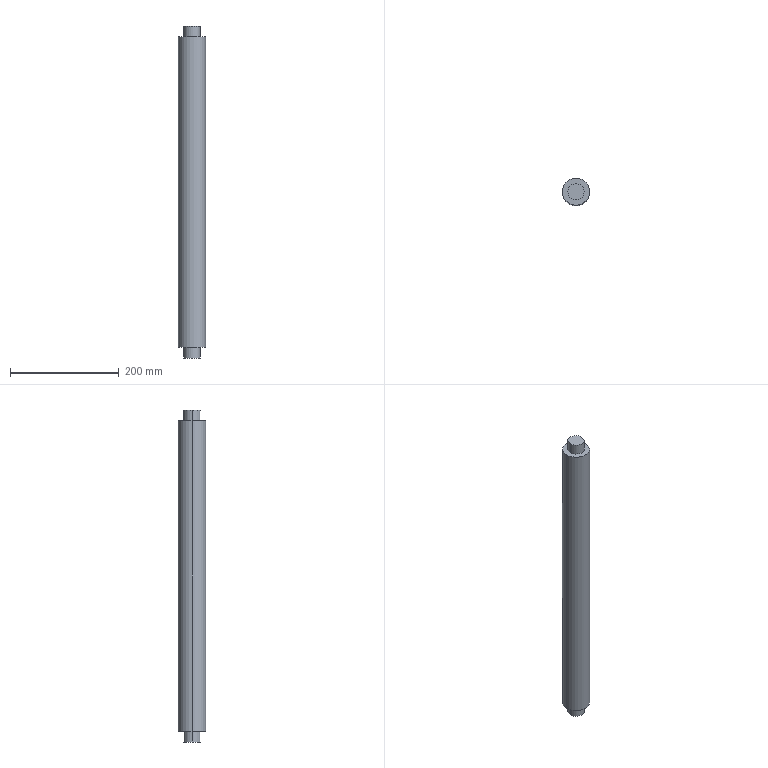Part | STEP file | 1 solid | 10 faces | box 50 x 50 x 610 mm | volume 1147467 mm3 | cylinder 6 | plane 4 | commonest cylinder face diameters 30 x4 50 x2
STEP:
#1=CARTESIAN_POINT('',(0.,0.,0.));
#2=DIRECTION('',(0.,0.,1.));
#3=DIRECTION('',(1.,0.,0.));
#4=AXIS2_PLACEMENT_3D('',#1,#2,#3);
#5=CARTESIAN_POINT('',(25.,0.,0.));
#6=VERTEX_POINT('',#5);
#7=CARTESIAN_POINT('',(-25.,0.,0.));
#8=VERTEX_POINT('',#7);
#9=CARTESIAN_POINT('',(0.,0.,0.));
#10=DIRECTION('',(0.,0.,1.));
#11=DIRECTION('',(1.,0.,0.));
#12=AXIS2_PLACEMENT_3D('',#9,#10,#11);
#13=CIRCLE('',#12,25.);
#14=CARTESIAN_POINT('',(0.,0.,0.));
#15=DIRECTION('',(0.,0.,1.));
#16=DIRECTION('',(1.,0.,0.));
#17=AXIS2_PLACEMENT_3D('',#14,#15,#16);
#18=CYLINDRICAL_SURFACE('',#17,25.);
#19=CARTESIAN_POINT('',(0.,0.));
#20=DIRECTION('',(1.,0.));
#21=VECTOR('',#20,1.);
#22=LINE('',#19,#21);
#23=(GEOMETRIC_REPRESENTATION_CONTEXT(2)PARAMETRIC_REPRESENTATION_CONTEXT()REPRESENTATION_CONTEXT('',''));
#24=DEFINITIONAL_REPRESENTATION('',(#22),#23);
#25=PCURVE('',#18,#24);
#26=CARTESIAN_POINT('',(0.,0.,0.));
#27=DIRECTION('',(0.,0.,1.));
#28=DIRECTION('',(1.,0.,0.));
#29=AXIS2_PLACEMENT_3D('',#26,#27,#28);
#30=PLANE('',#29);
#31=CARTESIAN_POINT('',(0.,0.));
#32=DIRECTION('',(1.,0.));
#33=AXIS2_PLACEMENT_2D('',#31,#32);
#34=CIRCLE('',#33,25.);
#35=(GEOMETRIC_REPRESENTATION_CONTEXT(2)PARAMETRIC_REPRESENTATION_CONTEXT()REPRESENTATION_CONTEXT('',''));
#36=DEFINITIONAL_REPRESENTATION('',(#34),#35);
#37=PCURVE('',#30,#36);
#38=SURFACE_CURVE('',#13,(#25,#37),.PCURVE_S1.);
#39=EDGE_CURVE('',#6,#8,#38,.T.);
#40=ORIENTED_EDGE('',*,*,#39,.T.);
#41=CARTESIAN_POINT('',(-25.,0.,570.));
#42=VERTEX_POINT('',#41);
#43=CARTESIAN_POINT('',(-25.,0.,0.));
#44=DIRECTION('',(0.,0.,1.));
#45=VECTOR('',#44,1.);
#46=LINE('',#43,#45);
#47=CARTESIAN_POINT('',(3.142,0.));
#48=DIRECTION('',(0.,1.));
#49=VECTOR('',#48,1.);
#50=LINE('',#47,#49);
#51=(GEOMETRIC_REPRESENTATION_CONTEXT(2)PARAMETRIC_REPRESENTATION_CONTEXT()REPRESENTATION_CONTEXT('',''));
#52=DEFINITIONAL_REPRESENTATION('',(#50),#51);
#53=PCURVE('',#18,#52);
#54=CARTESIAN_POINT('',(0.,0.,0.));
#55=DIRECTION('',(0.,0.,1.));
#56=DIRECTION('',(1.,0.,0.));
#57=AXIS2_PLACEMENT_3D('',#54,#55,#56);
#58=CYLINDRICAL_SURFACE('',#57,25.);
#59=CARTESIAN_POINT('',(3.142,0.));
#60=DIRECTION('',(0.,1.));
#61=VECTOR('',#60,1.);
#62=LINE('',#59,#61);
#63=(GEOMETRIC_REPRESENTATION_CONTEXT(2)PARAMETRIC_REPRESENTATION_CONTEXT()REPRESENTATION_CONTEXT('',''));
#64=DEFINITIONAL_REPRESENTATION('',(#62),#63);
#65=PCURVE('',#58,#64);
#66=SURFACE_CURVE('',#46,(#53,#65),.PCURVE_S1.);
#67=EDGE_CURVE('',#8,#42,#66,.T.);
#68=ORIENTED_EDGE('',*,*,#67,.T.);
#69=CARTESIAN_POINT('',(25.,0.,570.));
#70=VERTEX_POINT('',#69);
#71=CARTESIAN_POINT('',(0.,0.,570.));
#72=DIRECTION('',(0.,0.,-1.));
#73=DIRECTION('',(1.,0.,0.));
#74=AXIS2_PLACEMENT_3D('',#71,#72,#73);
#75=CIRCLE('',#74,25.);
#76=CARTESIAN_POINT('',(6.283,570.));
#77=DIRECTION('',(-1.,0.));
#78=VECTOR('',#77,1.);
#79=LINE('',#76,#78);
#80=(GEOMETRIC_REPRESENTATION_CONTEXT(2)PARAMETRIC_REPRESENTATION_CONTEXT()REPRESENTATION_CONTEXT('',''));
#81=DEFINITIONAL_REPRESENTATION('',(#79),#80);
#82=PCURVE('',#18,#81);
#83=CARTESIAN_POINT('',(0.,0.,570.));
#84=DIRECTION('',(0.,0.,1.));
#85=DIRECTION('',(1.,0.,0.));
#86=AXIS2_PLACEMENT_3D('',#83,#84,#85);
#87=PLANE('',#86);
#88=CARTESIAN_POINT('',(25.,0.));
#89=CARTESIAN_POINT('',(25.,-43.301));
#90=CARTESIAN_POINT('',(-12.5,-21.651));
#91=CARTESIAN_POINT('',(-50.,0.));
#92=CARTESIAN_POINT('',(-12.5,21.651));
#93=CARTESIAN_POINT('',(25.,43.301));
#94=CARTESIAN_POINT('',(25.,0.));
#95=(BOUNDED_CURVE()B_SPLINE_CURVE(2,(#88,#89,#90,#91,#92,#93,#94),.UNSPECIFIED.,.T.,.F.)B_SPLINE_CURVE_WITH_KNOTS((1,2,2,2,2,1),(-2.094,0.,2.094,4.189,6.283,8.378),.UNSPECIFIED.)CURVE()GEOMETRIC_REPRESENTATION_ITEM()RATIONAL_B_SPLINE_CURVE((1.,0.5,1.,0.5,1.,0.5,1.))REPRESENTATION_ITEM(''));
#96=(GEOMETRIC_REPRESENTATION_CONTEXT(2)PARAMETRIC_REPRESENTATION_CONTEXT()REPRESENTATION_CONTEXT('',''));
#97=DEFINITIONAL_REPRESENTATION('',(#95),#96);
#98=PCURVE('',#87,#97);
#99=SURFACE_CURVE('',#75,(#82,#98),.PCURVE_S1.);
#100=EDGE_CURVE('',#42,#70,#99,.T.);
#101=ORIENTED_EDGE('',*,*,#100,.T.);
#102=CARTESIAN_POINT('',(25.,0.,0.));
#103=DIRECTION('',(0.,0.,1.));
#104=VECTOR('',#103,1.);
#105=LINE('',#102,#104);
#106=CARTESIAN_POINT('',(0.,0.));
#107=DIRECTION('',(0.,1.));
#108=VECTOR('',#107,1.);
#109=LINE('',#106,#108);
#110=(GEOMETRIC_REPRESENTATION_CONTEXT(2)PARAMETRIC_REPRESENTATION_CONTEXT()REPRESENTATION_CONTEXT('',''));
#111=DEFINITIONAL_REPRESENTATION('',(#109),#110);
#112=PCURVE('',#18,#111);
#113=CARTESIAN_POINT('',(6.283,0.));
#114=DIRECTION('',(0.,1.));
#115=VECTOR('',#114,1.);
#116=LINE('',#113,#115);
#117=(GEOMETRIC_REPRESENTATION_CONTEXT(2)PARAMETRIC_REPRESENTATION_CONTEXT()REPRESENTATION_CONTEXT('',''));
#118=DEFINITIONAL_REPRESENTATION('',(#116),#117);
#119=PCURVE('',#58,#118);
#120=SURFACE_CURVE('',#105,(#112,#119),.PCURVE_S1.);
#121=EDGE_CURVE('',#6,#70,#120,.T.);
#122=ORIENTED_EDGE('',*,*,#121,.F.);
#123=EDGE_LOOP('',(#40,#68,#101,#122));
#124=FACE_BOUND('',#123,.T.);
#125=ADVANCED_FACE('',(#124),#18,.T.);
#126=CARTESIAN_POINT('',(-15.,0.,0.));
#127=VERTEX_POINT('',#126);
#128=CARTESIAN_POINT('',(15.,0.,0.));
#129=VERTEX_POINT('',#128);
#130=CARTESIAN_POINT('',(0.,0.,0.));
#131=DIRECTION('',(0.,0.,-1.));
#132=DIRECTION('',(-1.,0.,0.));
#133=AXIS2_PLACEMENT_3D('',#130,#131,#132);
#134=CIRCLE('',#133,15.);
#135=CARTESIAN_POINT('',(0.,0.,0.));
#136=DIRECTION('',(0.,0.,-1.));
#137=DIRECTION('',(-1.,0.,0.));
#138=AXIS2_PLACEMENT_3D('',#135,#136,#137);
#139=CYLINDRICAL_SURFACE('',#138,15.);
#140=CARTESIAN_POINT('',(0.,0.));
#141=DIRECTION('',(1.,0.));
#142=VECTOR('',#141,1.);
#143=LINE('',#140,#142);
#144=(GEOMETRIC_REPRESENTATION_CONTEXT(2)PARAMETRIC_REPRESENTATION_CONTEXT()REPRESENTATION_CONTEXT('',''));
#145=DEFINITIONAL_REPRESENTATION('',(#143),#144);
#146=PCURVE('',#139,#145);
#147=CARTESIAN_POINT('',(-15.,0.));
#148=CARTESIAN_POINT('',(-15.,25.981));
#149=CARTESIAN_POINT('',(7.5,12.99));
#150=CARTESIAN_POINT('',(30.,0.));
#151=CARTESIAN_POINT('',(7.5,-12.99));
#152=CARTESIAN_POINT('',(-15.,-25.981));
#153=CARTESIAN_POINT('',(-15.,0.));
#154=(BOUNDED_CURVE()B_SPLINE_CURVE(2,(#147,#148,#149,#150,#151,#152,#153),.UNSPECIFIED.,.T.,.F.)B_SPLINE_CURVE_WITH_KNOTS((1,2,2,2,2,1),(-2.094,0.,2.094,4.189,6.283,8.378),.UNSPECIFIED.)CURVE()GEOMETRIC_REPRESENTATION_ITEM()RATIONAL_B_SPLINE_CURVE((1.,0.5,1.,0.5,1.,0.5,1.))REPRESENTATION_ITEM(''));
#155=(GEOMETRIC_REPRESENTATION_CONTEXT(2)PARAMETRIC_REPRESENTATION_CONTEXT()REPRESENTATION_CONTEXT('',''));
#156=DEFINITIONAL_REPRESENTATION('',(#154),#155);
#157=PCURVE('',#30,#156);
#158=SURFACE_CURVE('',#134,(#146,#157),.PCURVE_S1.);
#159=EDGE_CURVE('',#127,#129,#158,.T.);
#160=ORIENTED_EDGE('',*,*,#159,.T.);
#161=CARTESIAN_POINT('',(15.,0.,-20.));
#162=VERTEX_POINT('',#161);
#163=CARTESIAN_POINT('',(15.,0.,0.));
#164=DIRECTION('',(0.,0.,-1.));
#165=VECTOR('',#164,1.);
#166=LINE('',#163,#165);
#167=CARTESIAN_POINT('',(3.142,0.));
#168=DIRECTION('',(0.,1.));
#169=VECTOR('',#168,1.);
#170=LINE('',#167,#169);
#171=(GEOMETRIC_REPRESENTATION_CONTEXT(2)PARAMETRIC_REPRESENTATION_CONTEXT()REPRESENTATION_CONTEXT('',''));
#172=DEFINITIONAL_REPRESENTATION('',(#170),#171);
#173=PCURVE('',#139,#172);
#174=CARTESIAN_POINT('',(0.,0.,0.));
#175=DIRECTION('',(0.,0.,-1.));
#176=DIRECTION('',(-1.,0.,0.));
#177=AXIS2_PLACEMENT_3D('',#174,#175,#176);
#178=CYLINDRICAL_SURFACE('',#177,15.);
#179=CARTESIAN_POINT('',(3.142,0.));
#180=DIRECTION('',(0.,1.));
#181=VECTOR('',#180,1.);
#182=LINE('',#179,#181);
#183=(GEOMETRIC_REPRESENTATION_CONTEXT(2)PARAMETRIC_REPRESENTATION_CONTEXT()REPRESENTATION_CONTEXT('',''));
#184=DEFINITIONAL_REPRESENTATION('',(#182),#183);
#185=PCURVE('',#178,#184);
#186=SURFACE_CURVE('',#166,(#173,#185),.PCURVE_S1.);
#187=EDGE_CURVE('',#129,#162,#186,.T.);
#188=ORIENTED_EDGE('',*,*,#187,.T.);
#189=CARTESIAN_POINT('',(-15.,0.,-20.));
#190=VERTEX_POINT('',#189);
#191=CARTESIAN_POINT('',(0.,0.,-20.));
#192=DIRECTION('',(0.,0.,1.));
#193=DIRECTION('',(-1.,0.,0.));
#194=AXIS2_PLACEMENT_3D('',#191,#192,#193);
#195=CIRCLE('',#194,15.);
#196=CARTESIAN_POINT('',(6.283,20.));
#197=DIRECTION('',(-1.,0.));
#198=VECTOR('',#197,1.);
#199=LINE('',#196,#198);
#200=(GEOMETRIC_REPRESENTATION_CONTEXT(2)PARAMETRIC_REPRESENTATION_CONTEXT()REPRESENTATION_CONTEXT('',''));
#201=DEFINITIONAL_REPRESENTATION('',(#199),#200);
#202=PCURVE('',#139,#201);
#203=CARTESIAN_POINT('',(0.,0.,-20.));
#204=DIRECTION('',(0.,0.,1.));
#205=DIRECTION('',(1.,0.,0.));
#206=AXIS2_PLACEMENT_3D('',#203,#204,#205);
#207=PLANE('',#206);
#208=CARTESIAN_POINT('',(0.,0.));
#209=DIRECTION('',(-1.,0.));
#210=AXIS2_PLACEMENT_2D('',#208,#209);
#211=CIRCLE('',#210,15.);
#212=(GEOMETRIC_REPRESENTATION_CONTEXT(2)PARAMETRIC_REPRESENTATION_CONTEXT()REPRESENTATION_CONTEXT('',''));
#213=DEFINITIONAL_REPRESENTATION('',(#211),#212);
#214=PCURVE('',#207,#213);
#215=SURFACE_CURVE('',#195,(#202,#214),.PCURVE_S1.);
#216=EDGE_CURVE('',#162,#190,#215,.T.);
#217=ORIENTED_EDGE('',*,*,#216,.T.);
#218=CARTESIAN_POINT('',(-15.,0.,0.));
#219=DIRECTION('',(0.,0.,-1.));
#220=VECTOR('',#219,1.);
#221=LINE('',#218,#220);
#222=CARTESIAN_POINT('',(0.,0.));
#223=DIRECTION('',(0.,1.));
#224=VECTOR('',#223,1.);
#225=LINE('',#222,#224);
#226=(GEOMETRIC_REPRESENTATION_CONTEXT(2)PARAMETRIC_REPRESENTATION_CONTEXT()REPRESENTATION_CONTEXT('',''));
#227=DEFINITIONAL_REPRESENTATION('',(#225),#226);
#228=PCURVE('',#139,#227);
#229=CARTESIAN_POINT('',(6.283,0.));
#230=DIRECTION('',(0.,1.));
#231=VECTOR('',#230,1.);
#232=LINE('',#229,#231);
#233=(GEOMETRIC_REPRESENTATION_CONTEXT(2)PARAMETRIC_REPRESENTATION_CONTEXT()REPRESENTATION_CONTEXT('',''));
#234=DEFINITIONAL_REPRESENTATION('',(#232),#233);
#235=PCURVE('',#178,#234);
#236=SURFACE_CURVE('',#221,(#228,#235),.PCURVE_S1.);
#237=EDGE_CURVE('',#127,#190,#236,.T.);
#238=ORIENTED_EDGE('',*,*,#237,.F.);
#239=EDGE_LOOP('',(#160,#188,#217,#238));
#240=FACE_BOUND('',#239,.T.);
#241=ADVANCED_FACE('',(#240),#139,.T.);
#242=CARTESIAN_POINT('',(-15.,0.,570.));
#243=VERTEX_POINT('',#242);
#244=CARTESIAN_POINT('',(15.,0.,570.));
#245=VERTEX_POINT('',#244);
#246=CARTESIAN_POINT('',(0.,0.,570.));
#247=DIRECTION('',(0.,0.,-1.));
#248=DIRECTION('',(1.,0.,0.));
#249=AXIS2_PLACEMENT_3D('',#246,#247,#248);
#250=CIRCLE('',#249,15.);
#251=CARTESIAN_POINT('',(0.,0.,570.));
#252=DIRECTION('',(0.,0.,1.));
#253=DIRECTION('',(1.,0.,0.));
#254=AXIS2_PLACEMENT_3D('',#251,#252,#253);
#255=CYLINDRICAL_SURFACE('',#254,15.);
#256=CARTESIAN_POINT('',(6.283,0.));
#257=DIRECTION('',(-1.,0.));
#258=VECTOR('',#257,1.);
#259=LINE('',#256,#258);
#260=(GEOMETRIC_REPRESENTATION_CONTEXT(2)PARAMETRIC_REPRESENTATION_CONTEXT()REPRESENTATION_CONTEXT('',''));
#261=DEFINITIONAL_REPRESENTATION('',(#259),#260);
#262=PCURVE('',#255,#261);
#263=CARTESIAN_POINT('',(15.,0.));
#264=CARTESIAN_POINT('',(15.,-25.981));
#265=CARTESIAN_POINT('',(-7.5,-12.99));
#266=CARTESIAN_POINT('',(-30.,0.));
#267=CARTESIAN_POINT('',(-7.5,12.99));
#268=CARTESIAN_POINT('',(15.,25.981));
#269=CARTESIAN_POINT('',(15.,0.));
#270=(BOUNDED_CURVE()B_SPLINE_CURVE(2,(#263,#264,#265,#266,#267,#268,#269),.UNSPECIFIED.,.T.,.F.)B_SPLINE_CURVE_WITH_KNOTS((1,2,2,2,2,1),(-2.094,0.,2.094,4.189,6.283,8.378),.UNSPECIFIED.)CURVE()GEOMETRIC_REPRESENTATION_ITEM()RATIONAL_B_SPLINE_CURVE((1.,0.5,1.,0.5,1.,0.5,1.))REPRESENTATION_ITEM(''));
#271=(GEOMETRIC_REPRESENTATION_CONTEXT(2)PARAMETRIC_REPRESENTATION_CONTEXT()REPRESENTATION_CONTEXT('',''));
#272=DEFINITIONAL_REPRESENTATION('',(#270),#271);
#273=PCURVE('',#87,#272);
#274=SURFACE_CURVE('',#250,(#262,#273),.PCURVE_S1.);
#275=EDGE_CURVE('',#243,#245,#274,.T.);
#276=ORIENTED_EDGE('',*,*,#275,.F.);
#277=CARTESIAN_POINT('',(-15.,0.,590.));
#278=VERTEX_POINT('',#277);
#279=CARTESIAN_POINT('',(-15.,0.,570.));
#280=DIRECTION('',(0.,0.,1.));
#281=VECTOR('',#280,1.);
#282=LINE('',#279,#281);
#283=CARTESIAN_POINT('',(3.142,0.));
#284=DIRECTION('',(0.,1.));
#285=VECTOR('',#284,1.);
#286=LINE('',#283,#285);
#287=(GEOMETRIC_REPRESENTATION_CONTEXT(2)PARAMETRIC_REPRESENTATION_CONTEXT()REPRESENTATION_CONTEXT('',''));
#288=DEFINITIONAL_REPRESENTATION('',(#286),#287);
#289=PCURVE('',#255,#288);
#290=CARTESIAN_POINT('',(0.,0.,570.));
#291=DIRECTION('',(0.,0.,1.));
#292=DIRECTION('',(1.,0.,0.));
#293=AXIS2_PLACEMENT_3D('',#290,#291,#292);
#294=CYLINDRICAL_SURFACE('',#293,15.);
#295=CARTESIAN_POINT('',(3.142,0.));
#296=DIRECTION('',(0.,1.));
#297=VECTOR('',#296,1.);
#298=LINE('',#295,#297);
#299=(GEOMETRIC_REPRESENTATION_CONTEXT(2)PARAMETRIC_REPRESENTATION_CONTEXT()REPRESENTATION_CONTEXT('',''));
#300=DEFINITIONAL_REPRESENTATION('',(#298),#299);
#301=PCURVE('',#294,#300);
#302=SURFACE_CURVE('',#282,(#289,#301),.PCURVE_S1.);
#303=EDGE_CURVE('',#243,#278,#302,.T.);
#304=ORIENTED_EDGE('',*,*,#303,.T.);
#305=CARTESIAN_POINT('',(15.,0.,590.));
#306=VERTEX_POINT('',#305);
#307=CARTESIAN_POINT('',(0.,0.,590.));
#308=DIRECTION('',(0.,0.,-1.));
#309=DIRECTION('',(1.,0.,0.));
#310=AXIS2_PLACEMENT_3D('',#307,#308,#309);
#311=CIRCLE('',#310,15.);
#312=CARTESIAN_POINT('',(6.283,20.));
#313=DIRECTION('',(-1.,0.));
#314=VECTOR('',#313,1.);
#315=LINE('',#312,#314);
#316=(GEOMETRIC_REPRESENTATION_CONTEXT(2)PARAMETRIC_REPRESENTATION_CONTEXT()REPRESENTATION_CONTEXT('',''));
#317=DEFINITIONAL_REPRESENTATION('',(#315),#316);
#318=PCURVE('',#255,#317);
#319=CARTESIAN_POINT('',(0.,0.,590.));
#320=DIRECTION('',(0.,0.,1.));
#321=DIRECTION('',(1.,0.,0.));
#322=AXIS2_PLACEMENT_3D('',#319,#320,#321);
#323=PLANE('',#322);
#324=CARTESIAN_POINT('',(15.,0.));
#325=CARTESIAN_POINT('',(15.,-25.981));
#326=CARTESIAN_POINT('',(-7.5,-12.99));
#327=CARTESIAN_POINT('',(-30.,0.));
#328=CARTESIAN_POINT('',(-7.5,12.99));
#329=CARTESIAN_POINT('',(15.,25.981));
#330=CARTESIAN_POINT('',(15.,0.));
#331=(BOUNDED_CURVE()B_SPLINE_CURVE(2,(#324,#325,#326,#327,#328,#329,#330),.UNSPECIFIED.,.T.,.F.)B_SPLINE_CURVE_WITH_KNOTS((1,2,2,2,2,1),(-2.094,0.,2.094,4.189,6.283,8.378),.UNSPECIFIED.)CURVE()GEOMETRIC_REPRESENTATION_ITEM()RATIONAL_B_SPLINE_CURVE((1.,0.5,1.,0.5,1.,0.5,1.))REPRESENTATION_ITEM(''));
#332=(GEOMETRIC_REPRESENTATION_CONTEXT(2)PARAMETRIC_REPRESENTATION_CONTEXT()REPRESENTATION_CONTEXT('',''));
#333=DEFINITIONAL_REPRESENTATION('',(#331),#332);
#334=PCURVE('',#323,#333);
#335=SURFACE_CURVE('',#311,(#318,#334),.PCURVE_S1.);
#336=EDGE_CURVE('',#278,#306,#335,.T.);
#337=ORIENTED_EDGE('',*,*,#336,.T.);
#338=CARTESIAN_POINT('',(15.,0.,570.));
#339=DIRECTION('',(0.,0.,1.));
#340=VECTOR('',#339,1.);
#341=LINE('',#338,#340);
#342=CARTESIAN_POINT('',(0.,0.));
#343=DIRECTION('',(0.,1.));
#344=VECTOR('',#343,1.);
#345=LINE('',#342,#344);
#346=(GEOMETRIC_REPRESENTATION_CONTEXT(2)PARAMETRIC_REPRESENTATION_CONTEXT()REPRESENTATION_CONTEXT('',''));
#347=DEFINITIONAL_REPRESENTATION('',(#345),#346);
#348=PCURVE('',#255,#347);
#349=CARTESIAN_POINT('',(6.283,0.));
#350=DIRECTION('',(0.,1.));
#351=VECTOR('',#350,1.);
#352=LINE('',#349,#351);
#353=(GEOMETRIC_REPRESENTATION_CONTEXT(2)PARAMETRIC_REPRESENTATION_CONTEXT()REPRESENTATION_CONTEXT('',''));
#354=DEFINITIONAL_REPRESENTATION('',(#352),#353);
#355=PCURVE('',#294,#354);
#356=SURFACE_CURVE('',#341,(#348,#355),.PCURVE_S1.);
#357=EDGE_CURVE('',#245,#306,#356,.T.);
#358=ORIENTED_EDGE('',*,*,#357,.F.);
#359=EDGE_LOOP('',(#276,#304,#337,#358));
#360=FACE_BOUND('',#359,.T.);
#361=ADVANCED_FACE('',(#360),#255,.T.);
#362=ORIENTED_EDGE('',*,*,#67,.F.);
#363=CARTESIAN_POINT('',(0.,0.,0.));
#364=DIRECTION('',(0.,0.,1.));
#365=DIRECTION('',(1.,0.,0.));
#366=AXIS2_PLACEMENT_3D('',#363,#364,#365);
#367=CIRCLE('',#366,25.);
#368=CARTESIAN_POINT('',(0.,0.));
#369=DIRECTION('',(1.,0.));
#370=VECTOR('',#369,1.);
#371=LINE('',#368,#370);
#372=(GEOMETRIC_REPRESENTATION_CONTEXT(2)PARAMETRIC_REPRESENTATION_CONTEXT()REPRESENTATION_CONTEXT('',''));
#373=DEFINITIONAL_REPRESENTATION('',(#371),#372);
#374=PCURVE('',#58,#373);
#375=CARTESIAN_POINT('',(0.,0.));
#376=DIRECTION('',(1.,0.));
#377=AXIS2_PLACEMENT_2D('',#375,#376);
#378=CIRCLE('',#377,25.);
#379=(GEOMETRIC_REPRESENTATION_CONTEXT(2)PARAMETRIC_REPRESENTATION_CONTEXT()REPRESENTATION_CONTEXT('',''));
#380=DEFINITIONAL_REPRESENTATION('',(#378),#379);
#381=PCURVE('',#30,#380);
#382=SURFACE_CURVE('',#367,(#374,#381),.PCURVE_S1.);
#383=EDGE_CURVE('',#8,#6,#382,.T.);
#384=ORIENTED_EDGE('',*,*,#383,.T.);
#385=ORIENTED_EDGE('',*,*,#121,.T.);
#386=CARTESIAN_POINT('',(0.,0.,570.));
#387=DIRECTION('',(0.,0.,-1.));
#388=DIRECTION('',(1.,0.,0.));
#389=AXIS2_PLACEMENT_3D('',#386,#387,#388);
#390=CIRCLE('',#389,25.);
#391=CARTESIAN_POINT('',(6.283,570.));
#392=DIRECTION('',(-1.,0.));
#393=VECTOR('',#392,1.);
#394=LINE('',#391,#393);
#395=(GEOMETRIC_REPRESENTATION_CONTEXT(2)PARAMETRIC_REPRESENTATION_CONTEXT()REPRESENTATION_CONTEXT('',''));
#396=DEFINITIONAL_REPRESENTATION('',(#394),#395);
#397=PCURVE('',#58,#396);
#398=CARTESIAN_POINT('',(25.,0.));
#399=CARTESIAN_POINT('',(25.,-43.301));
#400=CARTESIAN_POINT('',(-12.5,-21.651));
#401=CARTESIAN_POINT('',(-50.,0.));
#402=CARTESIAN_POINT('',(-12.5,21.651));
#403=CARTESIAN_POINT('',(25.,43.301));
#404=CARTESIAN_POINT('',(25.,0.));
#405=(BOUNDED_CURVE()B_SPLINE_CURVE(2,(#398,#399,#400,#401,#402,#403,#404),.UNSPECIFIED.,.T.,.F.)B_SPLINE_CURVE_WITH_KNOTS((1,2,2,2,2,1),(-2.094,0.,2.094,4.189,6.283,8.378),.UNSPECIFIED.)CURVE()GEOMETRIC_REPRESENTATION_ITEM()RATIONAL_B_SPLINE_CURVE((1.,0.5,1.,0.5,1.,0.5,1.))REPRESENTATION_ITEM(''));
#406=(GEOMETRIC_REPRESENTATION_CONTEXT(2)PARAMETRIC_REPRESENTATION_CONTEXT()REPRESENTATION_CONTEXT('',''));
#407=DEFINITIONAL_REPRESENTATION('',(#405),#406);
#408=PCURVE('',#87,#407);
#409=SURFACE_CURVE('',#390,(#397,#408),.PCURVE_S1.);
#410=EDGE_CURVE('',#70,#42,#409,.T.);
#411=ORIENTED_EDGE('',*,*,#410,.T.);
#412=EDGE_LOOP('',(#362,#384,#385,#411));
#413=FACE_BOUND('',#412,.T.);
#414=ADVANCED_FACE('',(#413),#58,.T.);
#415=ORIENTED_EDGE('',*,*,#39,.F.);
#416=ORIENTED_EDGE('',*,*,#383,.F.);
#417=EDGE_LOOP('',(#415,#416));
#418=FACE_BOUND('',#417,.T.);
#419=ORIENTED_EDGE('',*,*,#159,.F.);
#420=CARTESIAN_POINT('',(0.,0.,0.));
#421=DIRECTION('',(0.,0.,-1.));
#422=DIRECTION('',(-1.,0.,0.));
#423=AXIS2_PLACEMENT_3D('',#420,#421,#422);
#424=CIRCLE('',#423,15.);
#425=CARTESIAN_POINT('',(-15.,0.));
#426=CARTESIAN_POINT('',(-15.,25.981));
#427=CARTESIAN_POINT('',(7.5,12.99));
#428=CARTESIAN_POINT('',(30.,0.));
#429=CARTESIAN_POINT('',(7.5,-12.99));
#430=CARTESIAN_POINT('',(-15.,-25.981));
#431=CARTESIAN_POINT('',(-15.,0.));
#432=(BOUNDED_CURVE()B_SPLINE_CURVE(2,(#425,#426,#427,#428,#429,#430,#431),.UNSPECIFIED.,.T.,.F.)B_SPLINE_CURVE_WITH_KNOTS((1,2,2,2,2,1),(-2.094,0.,2.094,4.189,6.283,8.378),.UNSPECIFIED.)CURVE()GEOMETRIC_REPRESENTATION_ITEM()RATIONAL_B_SPLINE_CURVE((1.,0.5,1.,0.5,1.,0.5,1.))REPRESENTATION_ITEM(''));
#433=(GEOMETRIC_REPRESENTATION_CONTEXT(2)PARAMETRIC_REPRESENTATION_CONTEXT()REPRESENTATION_CONTEXT('',''));
#434=DEFINITIONAL_REPRESENTATION('',(#432),#433);
#435=PCURVE('',#30,#434);
#436=CARTESIAN_POINT('',(0.,0.));
#437=DIRECTION('',(1.,0.));
#438=VECTOR('',#437,1.);
#439=LINE('',#436,#438);
#440=(GEOMETRIC_REPRESENTATION_CONTEXT(2)PARAMETRIC_REPRESENTATION_CONTEXT()REPRESENTATION_CONTEXT('',''));
#441=DEFINITIONAL_REPRESENTATION('',(#439),#440);
#442=PCURVE('',#178,#441);
#443=SURFACE_CURVE('',#424,(#435,#442),.PCURVE_S1.);
#444=EDGE_CURVE('',#129,#127,#443,.T.);
#445=ORIENTED_EDGE('',*,*,#444,.F.);
#446=EDGE_LOOP('',(#419,#445));
#447=FACE_BOUND('',#446,.T.);
#448=ADVANCED_FACE('',(#418,#447),#30,.F.);
#449=ORIENTED_EDGE('',*,*,#410,.F.);
#450=ORIENTED_EDGE('',*,*,#100,.F.);
#451=EDGE_LOOP('',(#449,#450));
#452=FACE_BOUND('',#451,.T.);
#453=CARTESIAN_POINT('',(0.,0.,570.));
#454=DIRECTION('',(0.,0.,-1.));
#455=DIRECTION('',(1.,0.,0.));
#456=AXIS2_PLACEMENT_3D('',#453,#454,#455);
#457=CIRCLE('',#456,15.);
#458=CARTESIAN_POINT('',(15.,0.));
#459=CARTESIAN_POINT('',(15.,-25.981));
#460=CARTESIAN_POINT('',(-7.5,-12.99));
#461=CARTESIAN_POINT('',(-30.,0.));
#462=CARTESIAN_POINT('',(-7.5,12.99));
#463=CARTESIAN_POINT('',(15.,25.981));
#464=CARTESIAN_POINT('',(15.,0.));
#465=(BOUNDED_CURVE()B_SPLINE_CURVE(2,(#458,#459,#460,#461,#462,#463,#464),.UNSPECIFIED.,.T.,.F.)B_SPLINE_CURVE_WITH_KNOTS((1,2,2,2,2,1),(-2.094,0.,2.094,4.189,6.283,8.378),.UNSPECIFIED.)CURVE()GEOMETRIC_REPRESENTATION_ITEM()RATIONAL_B_SPLINE_CURVE((1.,0.5,1.,0.5,1.,0.5,1.))REPRESENTATION_ITEM(''));
#466=(GEOMETRIC_REPRESENTATION_CONTEXT(2)PARAMETRIC_REPRESENTATION_CONTEXT()REPRESENTATION_CONTEXT('',''));
#467=DEFINITIONAL_REPRESENTATION('',(#465),#466);
#468=PCURVE('',#87,#467);
#469=CARTESIAN_POINT('',(6.283,0.));
#470=DIRECTION('',(-1.,0.));
#471=VECTOR('',#470,1.);
#472=LINE('',#469,#471);
#473=(GEOMETRIC_REPRESENTATION_CONTEXT(2)PARAMETRIC_REPRESENTATION_CONTEXT()REPRESENTATION_CONTEXT('',''));
#474=DEFINITIONAL_REPRESENTATION('',(#472),#473);
#475=PCURVE('',#294,#474);
#476=SURFACE_CURVE('',#457,(#468,#475),.PCURVE_S1.);
#477=EDGE_CURVE('',#245,#243,#476,.T.);
#478=ORIENTED_EDGE('',*,*,#477,.T.);
#479=ORIENTED_EDGE('',*,*,#275,.T.);
#480=EDGE_LOOP('',(#478,#479));
#481=FACE_BOUND('',#480,.T.);
#482=ADVANCED_FACE('',(#452,#481),#87,.T.);
#483=ORIENTED_EDGE('',*,*,#187,.F.);
#484=ORIENTED_EDGE('',*,*,#444,.T.);
#485=ORIENTED_EDGE('',*,*,#237,.T.);
#486=CARTESIAN_POINT('',(0.,0.,-20.));
#487=DIRECTION('',(0.,0.,1.));
#488=DIRECTION('',(-1.,0.,0.));
#489=AXIS2_PLACEMENT_3D('',#486,#487,#488);
#490=CIRCLE('',#489,15.);
#491=CARTESIAN_POINT('',(6.283,20.));
#492=DIRECTION('',(-1.,0.));
#493=VECTOR('',#492,1.);
#494=LINE('',#491,#493);
#495=(GEOMETRIC_REPRESENTATION_CONTEXT(2)PARAMETRIC_REPRESENTATION_CONTEXT()REPRESENTATION_CONTEXT('',''));
#496=DEFINITIONAL_REPRESENTATION('',(#494),#495);
#497=PCURVE('',#178,#496);
#498=CARTESIAN_POINT('',(0.,0.));
#499=DIRECTION('',(-1.,0.));
#500=AXIS2_PLACEMENT_2D('',#498,#499);
#501=CIRCLE('',#500,15.);
#502=(GEOMETRIC_REPRESENTATION_CONTEXT(2)PARAMETRIC_REPRESENTATION_CONTEXT()REPRESENTATION_CONTEXT('',''));
#503=DEFINITIONAL_REPRESENTATION('',(#501),#502);
#504=PCURVE('',#207,#503);
#505=SURFACE_CURVE('',#490,(#497,#504),.PCURVE_S1.);
#506=EDGE_CURVE('',#190,#162,#505,.T.);
#507=ORIENTED_EDGE('',*,*,#506,.T.);
#508=EDGE_LOOP('',(#483,#484,#485,#507));
#509=FACE_BOUND('',#508,.T.);
#510=ADVANCED_FACE('',(#509),#178,.T.);
#511=ORIENTED_EDGE('',*,*,#303,.F.);
#512=ORIENTED_EDGE('',*,*,#477,.F.);
#513=ORIENTED_EDGE('',*,*,#357,.T.);
#514=CARTESIAN_POINT('',(0.,0.,590.));
#515=DIRECTION('',(0.,0.,-1.));
#516=DIRECTION('',(1.,0.,0.));
#517=AXIS2_PLACEMENT_3D('',#514,#515,#516);
#518=CIRCLE('',#517,15.);
#519=CARTESIAN_POINT('',(6.283,20.));
#520=DIRECTION('',(-1.,0.));
#521=VECTOR('',#520,1.);
#522=LINE('',#519,#521);
#523=(GEOMETRIC_REPRESENTATION_CONTEXT(2)PARAMETRIC_REPRESENTATION_CONTEXT()REPRESENTATION_CONTEXT('',''));
#524=DEFINITIONAL_REPRESENTATION('',(#522),#523);
#525=PCURVE('',#294,#524);
#526=CARTESIAN_POINT('',(15.,0.));
#527=CARTESIAN_POINT('',(15.,-25.981));
#528=CARTESIAN_POINT('',(-7.5,-12.99));
#529=CARTESIAN_POINT('',(-30.,0.));
#530=CARTESIAN_POINT('',(-7.5,12.99));
#531=CARTESIAN_POINT('',(15.,25.981));
#532=CARTESIAN_POINT('',(15.,0.));
#533=(BOUNDED_CURVE()B_SPLINE_CURVE(2,(#526,#527,#528,#529,#530,#531,#532),.UNSPECIFIED.,.T.,.F.)B_SPLINE_CURVE_WITH_KNOTS((1,2,2,2,2,1),(-2.094,0.,2.094,4.189,6.283,8.378),.UNSPECIFIED.)CURVE()GEOMETRIC_REPRESENTATION_ITEM()RATIONAL_B_SPLINE_CURVE((1.,0.5,1.,0.5,1.,0.5,1.))REPRESENTATION_ITEM(''));
#534=(GEOMETRIC_REPRESENTATION_CONTEXT(2)PARAMETRIC_REPRESENTATION_CONTEXT()REPRESENTATION_CONTEXT('',''));
#535=DEFINITIONAL_REPRESENTATION('',(#533),#534);
#536=PCURVE('',#323,#535);
#537=SURFACE_CURVE('',#518,(#525,#536),.PCURVE_S1.);
#538=EDGE_CURVE('',#306,#278,#537,.T.);
#539=ORIENTED_EDGE('',*,*,#538,.T.);
#540=EDGE_LOOP('',(#511,#512,#513,#539));
#541=FACE_BOUND('',#540,.T.);
#542=ADVANCED_FACE('',(#541),#294,.T.);
#543=ORIENTED_EDGE('',*,*,#506,.F.);
#544=ORIENTED_EDGE('',*,*,#216,.F.);
#545=EDGE_LOOP('',(#543,#544));
#546=FACE_BOUND('',#545,.T.);
#547=ADVANCED_FACE('',(#546),#207,.F.);
#548=ORIENTED_EDGE('',*,*,#538,.F.);
#549=ORIENTED_EDGE('',*,*,#336,.F.);
#550=EDGE_LOOP('',(#548,#549));
#551=FACE_BOUND('',#550,.T.);
#552=ADVANCED_FACE('',(#551),#323,.T.);
#553=CLOSED_SHELL('',(#125,#241,#361,#414,#448,#482,#510,#542,#547,#552));
#554=MANIFOLD_SOLID_BREP('',#553);
#555=(LENGTH_UNIT()NAMED_UNIT(*)SI_UNIT(.MILLI.,.METRE.));
#556=UNCERTAINTY_MEASURE_WITH_UNIT(LENGTH_MEASURE(0.0000001),#555,'','');
#557=(NAMED_UNIT(*)PLANE_ANGLE_UNIT()SI_UNIT($,.RADIAN.));
#558=(NAMED_UNIT(*)SI_UNIT($,.STERADIAN.)SOLID_ANGLE_UNIT());
#559=(GEOMETRIC_REPRESENTATION_CONTEXT(3)GLOBAL_UNCERTAINTY_ASSIGNED_CONTEXT((#556))GLOBAL_UNIT_ASSIGNED_CONTEXT((#555,#557,#558))REPRESENTATION_CONTEXT('',''));
#560=ADVANCED_BREP_SHAPE_REPRESENTATION('',(#4,#554),#559);